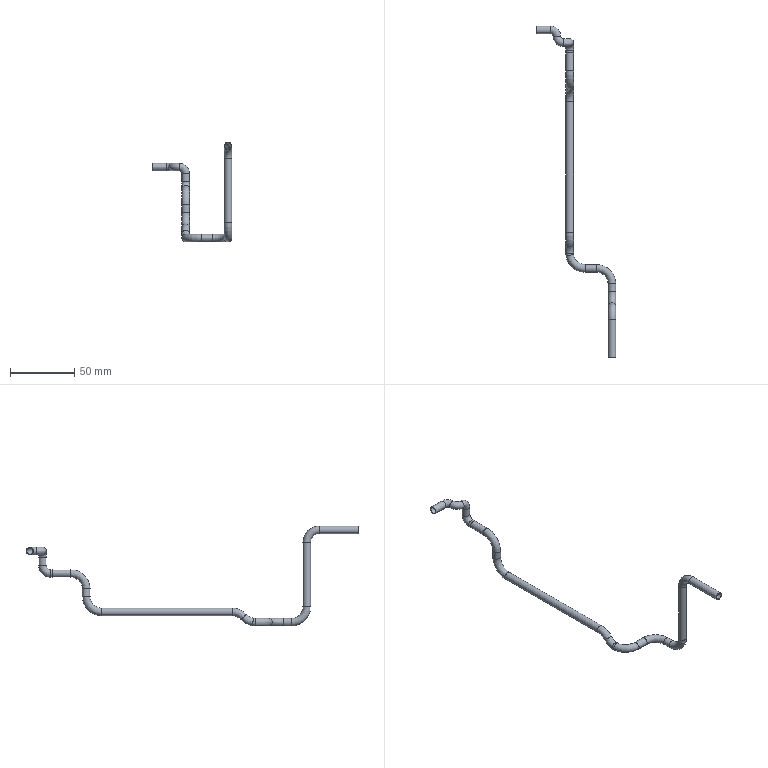Part | STEP file | 1-71 | 1 solid | 48 faces | box 62.108 x 259 x 78 mm | volume 3437 mm3 | torus 26 | cylinder 20 | plane 2 | commonest cylinder face diameters 5 x10 6 x10